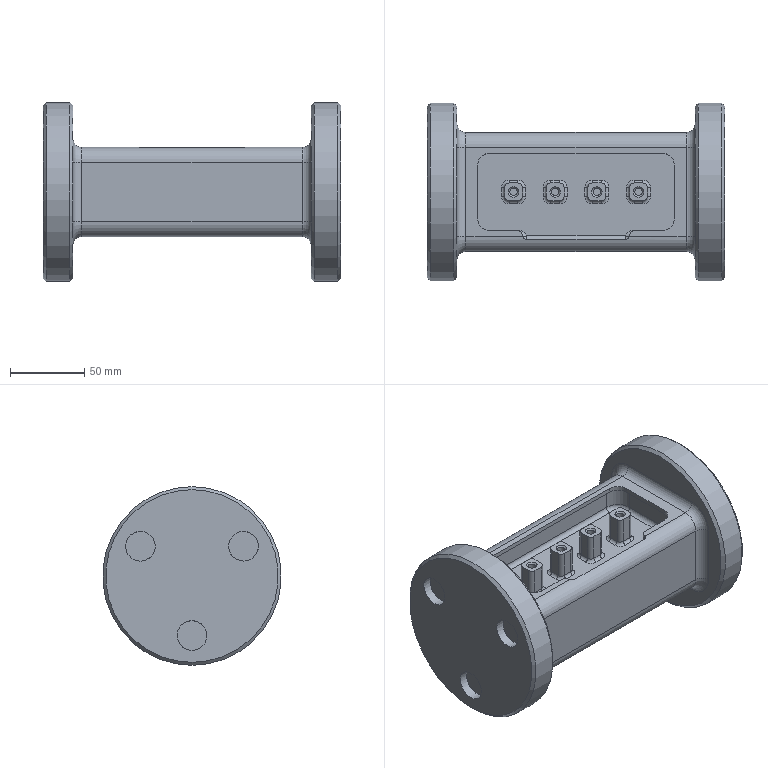NC program | NX | posted with a generic post | part box 200 x 120 x 120 mm
Lines 3125 to 4340 of 4340:
(CONTOUR_SURFACE_AREA , TOOL : PERSON_A_T_TOOL)
N6224 M6
N6226 G53
N6228 G17 G0 G90 X-24. Y-24. S3000 M3
N6230 G43 Z7. H0
N6232 Z1.
N6234 G94 G1 Z-9. F2500.
N6236 X-30.646
N6238 G3 X-38.875 Y-21. R11.134
N6240 G1 X-58.
N6242 G2 X-61. Y-18. R3.
N6244 G1 Y18.
N6246 G2 X-58. Y21. R3.
N6248 G1 X58.
N6250 G2 X61. Y18. R3.
N6252 G1 Y-18.
N6254 G2 X58. Y-21. R3.
N6256 G1 X38.875
N6258 G3 X30.646 Y-24. R11.134
N6260 G1 X24.
N6262 Z-9.367
N6264 X30.646
N6266 G2 X38.875 Y-21. R11.134
N6268 G1 X58.
N6270 G3 X61. Y-18. R3.
N6272 G1 Y18.
N6274 G3 X58. Y21. R3.
N6276 G1 X-58.
N6278 G3 X-61. Y18. R3.
N6280 G1 Y-18.
N6282 G3 X-58. Y-21. R3.
N6284 G1 X-38.875
N6286 G2 X-30.646 Y-24. R11.134
N6288 G1 X-24.
N6290 Z-9.733
N6292 X-30.646
N6294 G3 X-38.875 Y-21. R11.134
N6296 G1 X-58.
N6298 G2 X-61. Y-18. R3.
N6300 G1 Y18.
N6302 G2 X-58. Y21. R3.
N6304 G1 X58.
N6306 G2 X61. Y18. R3.
N6308 G1 Y-18.
N6310 G2 X58. Y-21. R3.
N6312 G1 X38.875
N6314 G3 X30.646 Y-24. R11.134
N6316 G1 X24.
N6318 Z-10.1
N6320 X30.646
N6322 G2 X38.875 Y-21. R11.134
N6324 G1 X58.
N6326 G3 X61. Y-18. R3.
N6328 G1 Y18.
N6330 G3 X58. Y21. R3.
N6332 G1 X-58.
N6334 G3 X-61. Y18. R3.
N6336 G1 Y-18.
N6338 G3 X-58. Y-21. R3.
N6340 G1 X-38.875
N6342 G2 X-30.646 Y-24. R11.134
N6344 G1 X-24.
N6346 Z-10.467
N6348 X-30.646
N6350 G3 X-38.875 Y-21. R11.134
N6352 G1 X-58.
N6354 G2 X-61. Y-18. R3.
N6356 G1 Y18.
N6358 G2 X-58. Y21. R3.
N6360 G1 X58.
N6362 G2 X61. Y18. R3.
N6364 G1 Y-18.
N6366 G2 X58. Y-21. R3.
N6368 G1 X38.875
N6370 G3 X30.646 Y-24. R11.134
N6372 G1 X24.
N6374 Z-10.833
N6376 X30.646
N6378 G2 X38.875 Y-21. R11.134
N6380 G1 X58.
N6382 G3 X61. Y-18. R3.
N6384 G1 Y18.
N6386 G3 X58. Y21. R3.
N6388 G1 X-58.
N6390 G3 X-61. Y18. R3.
N6392 G1 Y-18.
N6394 G3 X-58. Y-21. R3.
N6396 G1 X-38.875
N6398 G2 X-30.646 Y-24. R11.134
N6400 G1 X-24.
N6402 Z-11.2
N6404 X-30.646
N6406 G3 X-38.875 Y-21. R11.133
N6408 G1 X-58.
N6410 G2 X-61. Y-18. R3.
N6412 G1 Y18.
N6414 G2 X-58. Y21. R3.
N6416 G1 X58.
N6418 G2 X61. Y18. R3.
N6420 G1 Y-18.
N6422 G2 X58. Y-21. R3.
N6424 G1 X38.875
N6426 G3 X30.646 Y-24. R11.133
N6428 G1 X24.
N6430 Z-11.567
N6432 X30.646
N6434 G2 X38.875 Y-21. R11.133
N6436 G1 X58.
N6438 G3 X61. Y-18. R3.
N6440 G1 Y18.
N6442 G3 X58. Y21. R3.
N6444 G1 X-58.
N6446 G3 X-61. Y18. R3.
N6448 G1 Y-18.
N6450 G3 X-58. Y-21. R3.
N6452 G1 X-38.875
N6454 G2 X-30.646 Y-24. R11.134
N6456 G1 X-24.
N6458 Z-11.933
N6460 X-30.646
N6462 G3 X-38.875 Y-21. R11.134
N6464 G1 X-58.
N6466 G2 X-61. Y-18. R3.
N6468 G1 Y18.
N6470 G2 X-58. Y21. R3.
N6472 G1 X58.
N6474 G2 X61. Y18. R3.
N6476 G1 Y-18.
N6478 G2 X58. Y-21. R3.
N6480 G1 X38.875
N6482 G3 X30.646 Y-24. R11.134
N6484 G1 X24.
N6486 Z-12.3
N6488 X30.646
N6490 G2 X38.875 Y-21. R11.134
N6492 G1 X58.
N6494 G3 X61. Y-18. R3.
N6496 G1 Y18.
N6498 G3 X58. Y21. R3.
N6500 G1 X-58.
N6502 G3 X-61. Y18. R3.
N6504 G1 Y-18.
N6506 G3 X-58. Y-21. R3.
N6508 G1 X-38.875
N6510 G2 X-30.646 Y-24. R11.134
N6512 G1 X-24.
N6514 Z-12.667
N6516 X-30.646
N6518 G3 X-38.875 Y-21. R11.134
N6520 G1 X-58.
N6522 G2 X-61. Y-18. R3.
N6524 G1 Y18.
N6526 G2 X-58. Y21. R3.
N6528 G1 X58.
N6530 G2 X61. Y18. R3.
N6532 G1 Y-18.
N6534 G2 X58. Y-21. R3.
N6536 G1 X38.875
N6538 G3 X30.646 Y-24. R11.133
N6540 G1 X24.
N6542 Z-13.033
N6544 X30.646
N6546 G2 X38.875 Y-21. R11.134
N6548 G1 X58.
N6550 G3 X61. Y-18. R3.
N6552 G1 Y18.
N6554 G3 X58. Y21. R3.
N6556 G1 X-58.
N6558 G3 X-61. Y18. R3.
N6560 G1 Y-18.
N6562 G3 X-58. Y-21. R3.
N6564 G1 X-38.875
N6566 G2 X-30.646 Y-24. R11.134
N6568 G1 X-24.
N6570 Z-13.4
N6572 X-30.646
N6574 G3 X-38.875 Y-21. R11.133
N6576 G1 X-58.
N6578 G2 X-61. Y-18. R3.
N6580 G1 Y18.
N6582 G2 X-58. Y21. R3.
N6584 G1 X58.
N6586 G2 X61. Y18. R3.
N6588 G1 Y-18.
N6590 G2 X58. Y-21. R3.
N6592 G1 X38.875
N6594 G3 X30.646 Y-24. R11.133
N6596 G1 X24.
N6598 Z-13.767
N6600 X30.646
N6602 G2 X38.875 Y-21. R11.133
N6604 G1 X58.
N6606 G3 X61. Y-18. R3.
N6608 G1 Y18.
N6610 G3 X58. Y21. R3.
N6612 G1 X-58.
N6614 G3 X-61. Y18. R3.
N6616 G1 Y-18.
N6618 G3 X-58. Y-21. R3.
N6620 G1 X-38.875
N6622 G2 X-30.646 Y-24. R11.134
N6624 G1 X-24.
N6626 Z-14.133
N6628 X-30.646
N6630 G3 X-38.875 Y-21. R11.134
N6632 G1 X-58.
N6634 G2 X-61. Y-18. R3.
N6636 G1 Y18.
N6638 G2 X-58. Y21. R3.
N6640 G1 X58.
N6642 G2 X61. Y18. R3.
N6644 G1 Y-18.
N6646 G2 X58. Y-21. R3.
N6648 G1 X38.875
N6650 G3 X30.646 Y-24. R11.134
N6652 G1 X24.
N6654 Z-14.5
N6656 X30.646
N6658 G2 X38.875 Y-21. R11.134
N6660 G1 X58.
N6662 G3 X61. Y-18. R3.
N6664 G1 Y18.
N6666 G3 X58. Y21. R3.
N6668 G1 X-58.
N6670 G3 X-61. Y18. R3.
N6672 G1 Y-18.
N6674 G3 X-58. Y-21. R3.
N6676 G1 X-38.875
N6678 G2 X-30.646 Y-24. R11.134
N6680 G1 X-24.
N6682 Z-14.867
N6684 X-30.646
N6686 G3 X-38.875 Y-21. R11.134
N6688 G1 X-58.
N6690 G2 X-61. Y-18. R3.
N6692 G1 Y18.
N6694 G2 X-58. Y21. R3.
N6696 G1 X58.
N6698 G2 X61. Y18. R3.
N6700 G1 Y-18.
N6702 G2 X58. Y-21. R3.
N6704 G1 X38.875
N6706 G3 X30.646 Y-24. R11.134
N6708 G1 X24.
N6710 Z-15.233
N6712 X30.646
N6714 G2 X38.875 Y-21. R11.134
N6716 G1 X58.
N6718 G3 X61. Y-18. R3.
N6720 G1 Y18.
N6722 G3 X58. Y21. R3.
N6724 G1 X-58.
N6726 G3 X-61. Y18. R3.
N6728 G1 Y-18.
N6730 G3 X-58. Y-21. R3.
N6732 G1 X-38.875
N6734 G2 X-30.646 Y-24. R11.134
N6736 G1 X-24.
N6738 Z-15.6
N6740 X-30.646
N6742 G3 X-38.875 Y-21. R11.134
N6744 G1 X-58.
N6746 G2 X-61. Y-18. R3.
N6748 G1 Y18.
N6750 G2 X-58. Y21. R3.
N6752 G1 X58.
N6754 G2 X61. Y18. R3.
N6756 G1 Y-18.
N6758 G2 X58. Y-21. R3.
N6760 G1 X38.875
N6762 G3 X30.646 Y-24. R11.134
N6764 G1 X24.
N6766 Z-15.967
N6768 X30.646
N6770 G2 X38.875 Y-21. R11.134
N6772 G1 X58.
N6774 G3 X61. Y-18. R3.
N6776 G1 Y18.
N6778 G3 X58. Y21. R3.
N6780 G1 X-58.
N6782 G3 X-61. Y18. R3.
N6784 G1 Y-18.
N6786 G3 X-58. Y-21. R3.
N6788 G1 X-38.875
N6790 G2 X-30.646 Y-24. R11.134
N6792 G1 X-24.
N6794 Z-16.333
N6796 X-30.646
N6798 G3 X-38.875 Y-21. R11.134
N6800 G1 X-58.
N6802 G2 X-61. Y-18. R3.
N6804 G1 Y18.
N6806 G2 X-58. Y21. R3.
N6808 G1 X58.
N6810 G2 X61. Y18. R3.
N6812 G1 Y-18.
N6814 G2 X58. Y-21. R3.
N6816 G1 X38.875
N6818 G3 X30.646 Y-24. R11.134
N6820 G1 X24.
N6822 Z-16.7
N6824 X30.646
N6826 G2 X38.875 Y-21. R11.134
N6828 G1 X58.
N6830 G3 X61. Y-18. R3.
N6832 G1 Y18.
N6834 G3 X58. Y21. R3.
N6836 G1 X-58.
N6838 G3 X-61. Y18. R3.
N6840 G1 Y-18.
N6842 G3 X-58. Y-21. R3.
N6844 G1 X-38.875
N6846 G2 X-30.646 Y-24. R11.134
N6848 G1 X-24.
N6850 Y-23.999 Z-17.067
N6852 X-30.646
N6854 G3 X-38.875 Y-20.999 R11.134
N6856 G1 X-58.
N6858 G2 X-60.999 Y-18. R2.999
N6860 G1 Y18.
N6862 G2 X-58. Y20.999 R2.999
N6864 G1 X58.
N6866 G2 X60.999 Y18. R2.999
N6868 G1 Y-18.
N6870 G2 X58. Y-20.999 R2.999
N6872 G1 X38.875
N6874 G3 X30.646 Y-23.999 R11.134
N6876 G1 X24.
N6878 Y-23.969 Z-17.433
N6880 X30.634
N6882 G2 X38.875 Y-20.969 R11.165
N6884 G1 X58.
N6886 G3 X60.969 Y-18. R2.969
N6888 G1 Y18.
N6890 G3 X58. Y20.969 R2.969
N6892 G1 X-58.
N6894 G3 X-60.969 Y18. R2.969
N6896 G1 Y-18.
N6898 G3 X-58. Y-20.969 R2.969
N6900 G1 X-38.875
N6902 G2 X-30.634 Y-23.969 R11.165
N6904 G1 X-24.
N6906 Y-23.891 Z-17.8
N6908 X-30.603
N6910 G3 X-38.875 Y-20.891 R11.243
N6912 G1 X-58.
N6914 G2 X-60.891 Y-18. R2.891
N6916 G1 Y18.
N6918 G2 X-58. Y20.891 R2.891
N6920 G1 X58.
N6922 G2 X60.891 Y18. R2.891
N6924 G1 Y-18.
N6926 G2 X58. Y-20.891 R2.891
N6928 G1 X38.875
N6930 G3 X30.603 Y-23.891 R11.243
N6932 G1 X24.
N6934 Y-23.764 Z-18.167
N6936 X30.553
N6938 G2 X38.875 Y-20.764 R11.371
N6940 G1 X58.
N6942 G3 X60.764 Y-18. R2.764
N6944 G1 Y18.
N6946 G3 X58. Y20.764 R2.764
N6948 G1 X-58.
N6950 G3 X-60.764 Y18. R2.764
N6952 G1 Y-18.
N6954 G3 X-58. Y-20.764 R2.764
N6956 G1 X-38.875
N6958 G2 X-30.553 Y-23.764 R11.371
N6960 G1 X-24.
N6962 Y-23.679 Z-18.35
N6964 Y-23.579 Z-18.533
N6966 X-30.481
N6968 G3 X-38.875 Y-20.579 R11.558
N6970 G1 X-58.
N6972 G2 X-60.579 Y-18. R2.579
N6974 G1 Y18.
N6976 G2 X-58. Y20.579 R2.579
N6978 G1 X58.
N6980 G2 X60.579 Y18. R2.579
N6982 G1 Y-18.
N6984 G2 X58. Y-20.579 R2.579
N6986 G1 X38.875
N6988 G3 X30.481 Y-23.579 R11.558
N6990 G1 X24.
N6992 Y-23.46 Z-18.717
N6994 Y-23.322 Z-18.9
N6996 X30.381
N6998 G2 X38.875 Y-20.322 R11.816
N7000 G1 X58.
N7002 G3 X60.322 Y-18. R2.322
N7004 G1 Y18.
N7006 G3 X58. Y20.322 R2.322
N7008 G1 X-58.
N7010 G3 X-60.322 Y18. R2.322
N7012 G1 Y-18.
N7014 G3 X-58. Y-20.322 R2.322
N7016 G1 X-38.875
N7018 G2 X-30.381 Y-23.322 R11.816
N7020 G1 X-24.
N7022 Y-23.159 Z-19.083
N7024 Y-23.066 Z-19.175
N7026 Y-22.965 Z-19.267
N7028 X-30.246
N7030 G3 X-38.875 Y-19.965 R12.175
N7032 G1 X-58.
N7034 G2 X-59.965 Y-18. R1.965
N7036 G1 Y18.
N7038 G2 X-58. Y19.965 R1.965
N7040 G1 X58.
N7042 G2 X59.965 Y18. R1.965
N7044 G1 Y-18.
N7046 G2 X58. Y-19.965 R1.965
N7048 G1 X38.875
N7050 G3 X30.246 Y-22.965 R12.175
N7052 G1 X24.
N7054 Y-22.854 Z-19.358
N7056 Y-22.731 Z-19.45
N7058 Y-22.594 Z-19.542
N7060 Y-22.437 Z-19.633
N7062 X30.049
N7064 G2 X38.875 Y-19.437 R12.706
N7066 G1 X58.
N7068 G3 X59.437 Y-18. R1.437
N7070 G1 Y18.
N7072 G3 X58. Y19.437 R1.437
N7074 G1 X-58.
N7076 G3 X-59.437 Y18. R1.437
N7078 G1 Y-18.
N7080 G3 X-58. Y-19.437 R1.437
N7082 G1 X-38.875
N7084 G2 X-30.049 Y-22.437 R12.706
N7086 G1 X-24.
N7088 Y-22.35 Z-19.679
N7090 Y-22.255 Z-19.725
N7092 Y-22.033 Z-19.817
N7094 Y-21.736 Z-19.908
N7096 Y-21.522 Z-19.954
N7098 Y-21. Z-20.
N7100 X-28.25
N7102 X-29.313
N7104 X-29.578 Y-20.967
N7106 G3 X-36.75 Y-18.077 R14.082
N7108 G1 X-38.875 Y-18.
N7110 X-41. Y-18.005
N7112 X-49.5 Y-18.
N7114 X-53.75
N7116 X-55.875 Y-18.005
N7118 X-57.997 Y-17.998
N7120 X-57.998 Y-17.997
N7122 X-57.996 Y-17.998
N7124 X-57.998 Y-17.997
N7126 Y-17.998
N7128 X-57.991
N7130 X-57.988
N7132 X-57.987 Y-17.999
N7134 X-50.574 Y-18.
N7136 X-58. Y-17.965
N7138 Y9.
N7140 X-57.981 Y18.
N7142 X-57.987 Y17.999
N7144 X-57.991
N7146 X-57.993
N7148 X-57.998 Y17.998
N7150 X-57.996
N7152 X-57.998
N7154 X-57.997
N7156 X-57.998
N7158 Y17.991
N7160 X-58.
N7162 Y17.989
N7164 X-50.75 Y18.
N7166 X57.943
N7168 X57.999 Y17.993
N7170 X57.997 Y17.998
N7172 X57.998 Y17.996
N7174 X58. Y18.
N7176 X57.996 Y17.999
N7178 X57.998 Y17.997
N7180 X57.984 Y-17.999
N7182 X57.988 Y-17.998
N7184 X57.991
N7186 X57.998
N7188 X57.995
N7190 X57.998
N7192 Y-17.995
N7194 X57.997 Y-17.998
N7196 X57.998
N7198 Y-17.991
N7200 Y-17.988
N7202 X57.999 Y-17.984
N7204 X58. Y-17.911
N7206 X53.75 Y-18.
N7208 X49.5
N7210 X41. Y-18.005
N7212 X38.875 Y-18.
N7214 X36.75 Y-18.077
N7216 G3 X29.578 Y-20.967 R14.05
N7218 G1 X29.313 Y-21.
N7220 X24.
N7222 Z-17.
N7224 G0 Z7.
(CONTOUR_SURFACE_AREA_COPY , TOOL : PERSON_A_T_TOOL)
N7226 X-24. Y-26.
N7228 Z1.
N7230 Z-8.7
N7232 G1 Z-9.
N7234 X-58.
N7236 G2 X-66. Y-18. R8.
N7238 G1 Y18.
N7240 G2 X-58. Y26. R8.
N7242 G1 X58.
N7244 G2 X66. Y18. R8.
N7246 G1 Y-18.
N7248 G2 X58. Y-26. R8.
N7250 G1 X24.
N7252 Z-10.1
N7254 X58.
N7256 G3 X66. Y-18. R8.
N7258 G1 Y18.
N7260 G3 X58. Y26. R8.
N7262 G1 X-58.
N7264 G3 X-66. Y18. R8.
N7266 G1 Y-18.
N7268 G3 X-58. Y-26. R8.
N7270 G1 X-24.
N7272 Z-11.2
N7274 X-58.
N7276 G2 X-66. Y-18. R8.
N7278 G1 Y18.
N7280 G2 X-58. Y26. R8.
N7282 G1 X58.
N7284 G2 X66. Y18. R8.
N7286 G1 Y-18.
N7288 G2 X58. Y-26. R8.
N7290 G1 X24.
N7292 Z-12.3
N7294 X58.
N7296 G3 X66. Y-18. R8.
N7298 G1 Y18.
N7300 G3 X58. Y26. R8.
N7302 G1 X-58.
N7304 G3 X-66. Y18. R8.
N7306 G1 Y-18.
N7308 G3 X-58. Y-26. R8.
N7310 G1 X-24.
N7312 Z-13.4
N7314 X-58.
N7316 G2 X-66. Y-18. R8.
N7318 G1 Y18.
N7320 G2 X-58. Y26. R8.
N7322 G1 X58.
N7324 G2 X66. Y18. R8.
N7326 G1 Y-18.
N7328 G2 X58. Y-26. R8.
N7330 G1 X24.
N7332 Z-14.5
N7334 X58.
N7336 G3 X66. Y-18. R8.
N7338 G1 Y18.
N7340 G3 X58. Y26. R8.
N7342 G1 X-58.
N7344 G3 X-66. Y18. R8.
N7346 G1 Y-18.
N7348 G3 X-58. Y-26. R8.
N7350 G1 X-24.
N7352 Z-15.6
N7354 X-58.
N7356 G2 X-66. Y-18. R8.
N7358 G1 Y18.
N7360 G2 X-58. Y26. R8.
N7362 G1 X58.
N7364 G2 X66. Y18. R8.
N7366 G1 Y-18.
N7368 G2 X58. Y-26. R8.
N7370 G1 X24.
N7372 Z-16.7
N7374 X58.
N7376 G3 X66. Y-18. R8.
N7378 G1 Y18.
N7380 G3 X58. Y26. R8.
N7382 G1 X-58.
N7384 G3 X-66. Y18. R8.
N7386 G1 Y-18.
N7388 G3 X-58. Y-26. R8.
N7390 G1 X-24.
N7392 Z-17.8
N7394 X-58.
N7396 G2 X-66. Y-18. R8.
N7398 G1 Y18.
N7400 G2 X-58. Y26. R8.
N7402 G1 X58.
N7404 G2 X66. Y18. R8.
N7406 G1 Y-18.
N7408 G2 X58. Y-26. R8.
N7410 G1 X24.
N7412 Z-18.9
N7414 X58.
N7416 G3 X66. Y-18. R8.
N7418 G1 Y18.
N7420 G3 X58. Y26. R8.
N7422 G1 X-58.
N7424 G3 X-66. Y18. R8.
N7426 G1 Y-18.
N7428 G3 X-58. Y-26. R8.
N7430 G1 X-24.
N7432 Z-20.
N7434 X-58.
N7436 G2 X-66. Y-18. R8.
N7438 G1 Y18.
N7440 G2 X-58. Y26. R8.
N7442 G1 X58.
N7444 G2 X66. Y18. R8.
N7446 G1 Y-18.
N7448 G2 X58. Y-26. R8.
N7450 G1 X24.
N7452 Z-19.7
N7454 G0 Z1.
(CONTOUR_SURFACE_AREA_COPY_1 , TOOL : PERSON_A_T_TOOL)
N7456 Z7.
N7458 X-24. Y-24.
N7460 Z1.
N7462 G1 Z-9.
N7464 X-30.646
N7466 G3 X-38.875 Y-21. R11.134
N7468 G1 X-58.
N7470 G2 X-61. Y-18. R3.
N7472 G1 Y18.
N7474 G2 X-58. Y21. R3.
N7476 G1 X58.
N7478 G2 X61. Y18. R3.
N7480 G1 Y-18.
N7482 G2 X58. Y-21. R3.
N7484 G1 X38.875
N7486 G3 X30.646 Y-24. R11.134
N7488 G1 X24.
N7490 Z-10.54
N7492 X30.646
N7494 G2 X38.875 Y-21. R11.134
N7496 G1 X58.
N7498 G3 X61. Y-18. R3.
N7500 G1 Y18.
N7502 G3 X58. Y21. R3.
N7504 G1 X-58.
N7506 G3 X-61. Y18. R3.
N7508 G1 Y-18.
N7510 G3 X-58. Y-21. R3.
N7512 G1 X-38.875
N7514 G2 X-30.646 Y-24. R11.134
N7516 G1 X-24.
N7518 Z-12.08
N7520 X-30.646
N7522 G3 X-38.875 Y-21. R11.133
N7524 G1 X-58.
N7526 G2 X-61. Y-18. R3.
N7528 G1 Y18.
N7530 G2 X-58. Y21. R3.
N7532 G1 X58.
N7534 G2 X61. Y18. R3.
N7536 G1 Y-18.
N7538 G2 X58. Y-21. R3.
N7540 G1 X38.875
N7542 G3 X30.646 Y-24. R11.134
N7544 G1 X24.
N7546 Z-13.62
N7548 X30.646
N7550 G2 X38.875 Y-21. R11.134
N7552 G1 X58.
N7554 G3 X61. Y-18. R3.
N7556 G1 Y18.
N7558 G3 X58. Y21. R3.
N7560 G1 X-58.
N7562 G3 X-61. Y18. R3.
N7564 G1 Y-18.
N7566 G3 X-58. Y-21. R3.
N7568 G1 X-38.875
N7570 G2 X-30.646 Y-24. R11.134
N7572 G1 X-24.
N7574 Z-15.16
N7576 X-30.646
N7578 G3 X-38.875 Y-21. R11.134
N7580 G1 X-58.
N7582 G2 X-61. Y-18. R3.
N7584 G1 Y18.
N7586 G2 X-58. Y21. R3.
N7588 G1 X58.
N7590 G2 X61. Y18. R3.
N7592 G1 Y-18.
N7594 G2 X58. Y-21. R3.
N7596 G1 X38.875
N7598 G3 X30.646 Y-24. R11.134
N7600 G1 X24.
N7602 Z-16.7
N7604 X30.646
N7606 G2 X38.875 Y-21. R11.134
N7608 G1 X58.
N7610 G3 X61. Y-18. R3.
N7612 G1 Y18.
N7614 G3 X58. Y21. R3.
N7616 G1 X-58.
N7618 G3 X-61. Y18. R3.
N7620 G1 Y-18.
N7622 G3 X-58. Y-21. R3.
N7624 G1 X-38.875
N7626 G2 X-30.646 Y-24. R11.134
N7628 G1 X-24.
N7630 Z1.
N7632 G0 Z7.
(CONTOUR_SURFACE_AREA_COPY_1_COPY , TOOL : PERSON_A_T_TOOL)
N7634 Z1.
N7636 G1 Z-16.7
N7638 X-30.646
N7640 G3 X-38.875 Y-21. R11.134
N7642 G1 X-58.
N7644 G2 X-61. Y-18. R3.
N7646 G1 Y18.
N7648 G2 X-58. Y21. R3.
N7650 G1 X58.
N7652 G2 X61. Y18. R3.
N7654 G1 Y-18.
N7656 G2 X58. Y-21. R3.
N7658 G1 X38.875
N7660 G3 X30.646 Y-24. R11.134
N7662 G1 X24.
N7664 Z-16.81
N7666 X30.646
N7668 G2 X38.875 Y-21. R11.134
N7670 G1 X58.
N7672 G3 X61. Y-18. R3.
N7674 G1 Y18.
N7676 G3 X58. Y21. R3.
N7678 G1 X-58.
N7680 G3 X-61. Y18. R3.
N7682 G1 Y-18.
N7684 G3 X-58. Y-21. R3.
N7686 G1 X-38.875
N7688 G2 X-30.646 Y-24. R11.134
N7690 G1 X-24.
N7692 Z-16.92
N7694 X-30.646
N7696 G3 X-38.875 Y-21. R11.134
N7698 G1 X-58.
N7700 G2 X-61. Y-18. R3.
N7702 G1 Y18.
N7704 G2 X-58. Y21. R3.
N7706 G1 X58.
N7708 G2 X61. Y18. R3.
N7710 G1 Y-18.
N7712 G2 X58. Y-21. R3.
N7714 G1 X38.875
N7716 G3 X30.646 Y-24. R11.134
N7718 G1 X24.
N7720 Z-17.03
N7722 X30.646
N7724 G2 X38.875 Y-21. R11.134
N7726 G1 X58.
N7728 G3 X61. Y-18. R3.
N7730 G1 Y18.
N7732 G3 X58. Y21. R3.
N7734 G1 X-58.
N7736 G3 X-61. Y18. R3.
N7738 G1 Y-18.
N7740 G3 X-58. Y-21. R3.
N7742 G1 X-38.875
N7744 G2 X-30.646 Y-24. R11.134
N7746 G1 X-24.
N7748 Y-23.997 Z-17.14
N7750 X-30.645
N7752 G3 X-38.875 Y-20.997 R11.137
N7754 G1 X-58.
N7756 G2 X-60.997 Y-18. R2.997
N7758 G1 Y18.
N7760 G2 X-58. Y20.997 R2.997
N7762 G1 X58.
N7764 G2 X60.997 Y18. R2.997
N7766 G1 Y-18.
N7768 G2 X58. Y-20.997 R2.997
N7770 G1 X38.875
N7772 G3 X30.645 Y-23.997 R11.137
N7774 G1 X24.
N7776 Y-23.99 Z-17.25
N7778 X30.633
N7780 G2 X38.875 Y-20.99 R11.18
N7782 G1 X58.
N7784 G3 X60.99 Y-18. R2.99
N7786 G1 Y18.
N7788 G3 X58. Y20.99 R2.99
N7790 G1 X-58.
N7792 G3 X-60.99 Y18. R2.99
N7794 G1 Y-18.
N7796 G3 X-58. Y-20.99 R2.99
N7798 G1 X-38.875
N7800 G2 X-30.633 Y-23.99 R11.18
N7802 G1 X-24.
N7804 Y-23.978 Z-17.36
N7806 X-30.638
N7808 G3 X-38.875 Y-20.978 R11.155
N7810 G1 X-58.
N7812 G2 X-60.978 Y-18. R2.978
N7814 G1 Y18.
N7816 G2 X-58. Y20.978 R2.978
N7818 G1 X58.
N7820 G2 X60.978 Y18. R2.978
N7822 G1 Y-18.
N7824 G2 X58. Y-20.978 R2.978
N7826 G1 X38.875
N7828 G3 X30.638 Y-23.978 R11.155
N7830 G1 X24.
N7832 Y-23.963 Z-17.47
N7834 X30.632
N7836 G2 X38.875 Y-20.963 R11.171
N7838 G1 X58.
N7840 G3 X60.963 Y-18. R2.963
N7842 G1 Y18.
N7844 G3 X58. Y20.963 R2.963
N7846 G1 X-58.
N7848 G3 X-60.963 Y18. R2.963
N7850 G1 Y-18.
N7852 G3 X-58. Y-20.963 R2.963
N7854 G1 X-38.875
N7856 G2 X-30.632 Y-23.963 R11.171
N7858 G1 X-24.
N7860 Y-23.943 Z-17.58
N7862 X-30.624
N7864 G3 X-38.875 Y-20.943 R11.191
N7866 G1 X-58.
N7868 G2 X-60.943 Y-18. R2.943
N7870 G1 Y18.
N7872 G2 X-58. Y20.943 R2.943
N7874 G1 X58.
N7876 G2 X60.943 Y18. R2.943
N7878 G1 Y-18.
N7880 G2 X58. Y-20.943 R2.943
N7882 G1 X38.875
N7884 G3 X30.624 Y-23.943 R11.191
N7886 G1 X24.
N7888 Y-23.92 Z-17.69
N7890 X30.614
N7892 G2 X38.875 Y-20.92 R11.214
N7894 G1 X58.
N7896 G3 X60.92 Y-18. R2.92
N7898 G1 Y18.
N7900 G3 X58. Y20.92 R2.92
N7902 G1 X-58.
N7904 G3 X-60.92 Y18. R2.92
N7906 G1 Y-18.
N7908 G3 X-58. Y-20.92 R2.92
N7910 G1 X-38.875
N7912 G2 X-30.614 Y-23.92 R11.214
N7914 G1 X-24.
N7916 Y-23.891 Z-17.8
N7918 X-30.603
N7920 G3 X-38.875 Y-20.891 R11.243
N7922 G1 X-58.
N7924 G2 X-60.891 Y-18. R2.891
N7926 G1 Y18.
N7928 G2 X-58. Y20.891 R2.891
N7930 G1 X58.
N7932 G2 X60.891 Y18. R2.891
N7934 G1 Y-18.
N7936 G2 X58. Y-20.891 R2.891
N7938 G1 X38.875
N7940 G3 X30.603 Y-23.891 R11.243
N7942 G1 X24.
N7944 Y-23.859 Z-17.91
N7946 X30.59
N7948 G2 X38.875 Y-20.859 R11.276
N7950 G1 X58.
N7952 G3 X60.859 Y-18. R2.859
N7954 G1 Y18.
N7956 G3 X58. Y20.859 R2.859
N7958 G1 X-58.
N7960 G3 X-60.859 Y18. R2.859
N7962 G1 Y-18.
N7964 G3 X-58. Y-20.859 R2.859
N7966 G1 X-38.875
N7968 G2 X-30.59 Y-23.859 R11.276
N7970 G1 X-24.
N7972 Y-23.821 Z-18.02
N7974 X-30.575
N7976 G3 X-38.875 Y-20.821 R11.315
N7978 G1 X-58.
N7980 G2 X-60.821 Y-18. R2.821
N7982 G1 Y18.
N7984 G2 X-58. Y20.821 R2.821
N7986 G1 X58.
N7988 G2 X60.821 Y18. R2.821
N7990 G1 Y-18.
N7992 G2 X58. Y-20.821 R2.821
N7994 G1 X38.875
N7996 G3 X30.575 Y-23.821 R11.315
N7998 G1 X24.
N8000 Y-23.779 Z-18.13
N8002 X30.559
N8004 G2 X38.875 Y-20.779 R11.356
N8006 G1 X58.
N8008 G3 X60.779 Y-18. R2.779
N8010 G1 Y18.
N8012 G3 X58. Y20.779 R2.779
N8014 G1 X-58.
N8016 G3 X-60.779 Y18. R2.779
N8018 G1 Y-18.
N8020 G3 X-58. Y-20.779 R2.779
N8022 G1 X-38.875
N8024 G2 X-30.559 Y-23.779 R11.356
N8026 G1 X-24.
N8028 Y-23.732 Z-18.24
N8030 X-30.54
N8032 G3 X-38.875 Y-20.732 R11.404
N8034 G1 X-58.
N8036 G2 X-60.732 Y-18. R2.732
N8038 G1 Y18.
N8040 G2 X-58. Y20.732 R2.732
N8042 G1 X58.
N8044 G2 X60.732 Y18. R2.732
N8046 G1 Y-18.
N8048 G2 X58. Y-20.732 R2.732
N8050 G1 X38.875
N8052 G3 X30.54 Y-23.732 R11.404
N8054 G1 X24.
N8056 Y-23.679 Z-18.35
N8058 X30.52
N8060 G2 X38.875 Y-20.679 R11.457
N8062 G1 X58.
N8064 G3 X60.679 Y-18. R2.679
N8066 G1 Y18.
N8068 G3 X58. Y20.679 R2.679
N8070 G1 X-58.
N8072 G3 X-60.679 Y18. R2.679
N8074 G1 Y-18.
N8076 G3 X-58. Y-20.679 R2.679
N8078 G1 X-38.875
N8080 G2 X-30.52 Y-23.679 R11.457
N8082 G1 X-24.
N8084 Y-23.621 Z-18.46
N8086 X-30.497
N8088 G3 X-38.875 Y-20.621 R11.515
N8090 G1 X-58.
N8092 G2 X-60.621 Y-18. R2.621
N8094 G1 Y18.
N8096 G2 X-58. Y20.621 R2.621
N8098 G1 X58.
N8100 G2 X60.621 Y18. R2.621
N8102 G1 Y-18.
N8104 G2 X58. Y-20.621 R2.621
N8106 G1 X38.875
N8108 G3 X30.497 Y-23.621 R11.515
N8110 G1 X24.
N8112 Y-23.556 Z-18.57
N8114 X30.472
N8116 G2 X38.875 Y-20.556 R11.581
N8118 G1 X58.
N8120 G3 X60.556 Y-18. R2.556
N8122 G1 Y18.
N8124 G3 X58. Y20.556 R2.556
N8126 G1 X-58.
N8128 G3 X-60.556 Y18. R2.556
N8130 G1 Y-18.
N8132 G3 X-58. Y-20.556 R2.556
N8134 G1 X-38.875
N8136 G2 X-30.472 Y-23.556 R11.581
N8138 G1 X-24.
N8140 Y-23.485 Z-18.68
N8142 X-30.445
N8144 G3 X-38.875 Y-20.485 R11.651
N8146 G1 X-58.
N8148 G2 X-60.485 Y-18. R2.485
N8150 G1 Y18.
N8152 G2 X-58. Y20.485 R2.485
N8154 G1 X58.
N8156 G2 X60.485 Y18. R2.485
N8158 G1 Y-18.
N8160 G2 X58. Y-20.485 R2.485
N8162 G1 X38.875
N8164 G3 X30.445 Y-23.485 R11.651
N8166 G1 X24.
N8168 Y-23.407 Z-18.79
N8170 X30.414
N8172 G2 X38.875 Y-20.407 R11.73
N8174 G1 X58.
N8176 G3 X60.407 Y-18. R2.407
N8178 G1 Y18.
N8180 G3 X58. Y20.407 R2.407
N8182 G1 X-58.
N8184 G3 X-60.407 Y18. R2.407
N8186 G1 Y-18.
N8188 G3 X-58. Y-20.407 R2.407
N8190 G1 X-38.875
N8192 G2 X-30.414 Y-23.407 R11.73
N8194 G1 X-24.
N8196 Y-23.322 Z-18.9
N8198 X-30.381
N8200 G3 X-38.875 Y-20.322 R11.816
N8202 G1 X-58.
N8204 G2 X-60.322 Y-18. R2.322
N8206 G1 Y18.
N8208 G2 X-58. Y20.322 R2.322
N8210 G1 X58.
N8212 G2 X60.322 Y18. R2.322
N8214 G1 Y-18.
N8216 G2 X58. Y-20.322 R2.322
N8218 G1 X38.875
N8220 G3 X30.381 Y-23.322 R11.816
N8222 G1 X24.
N8224 Y-23.227 Z-19.01
N8226 X30.345
N8228 G2 X38.875 Y-20.227 R11.911
N8230 G1 X58.
N8232 G3 X60.227 Y-18. R2.227
N8234 G1 Y18.
N8236 G3 X58. Y20.227 R2.227
N8238 G1 X-58.
N8240 G3 X-60.227 Y18. R2.227
N8242 G1 Y-18.
N8244 G3 X-58. Y-20.227 R2.227
N8246 G1 X-38.875
N8248 G2 X-30.345 Y-23.227 R11.911
N8250 G1 X-24.
N8252 Y-23.123 Z-19.12
N8254 X-30.305
N8256 G3 X-38.875 Y-20.123 R12.017
N8258 G1 X-58.
N8260 G2 X-60.123 Y-18. R2.123
N8262 G1 Y18.
N8264 G2 X-58. Y20.123 R2.123
N8266 G1 X58.
N8268 G2 X60.123 Y18. R2.123
N8270 G1 Y-18.
N8272 G2 X58. Y-20.123 R2.123
N8274 G1 X38.875
N8276 G3 X30.305 Y-23.123 R12.017
N8278 G1 X24.
N8280 Y-23.007 Z-19.23
N8282 X30.261
N8284 G2 X38.875 Y-20.007 R12.133
N8286 G1 X58.
N8288 G3 X60.007 Y-18. R2.007
N8290 G1 Y18.
N8292 G3 X58. Y20.007 R2.007
N8294 G1 X-58.
N8296 G3 X-60.007 Y18. R2.007
N8298 G1 Y-18.
N8300 G3 X-58. Y-20.007 R2.007
N8302 G1 X-38.875
N8304 G2 X-30.261 Y-23.007 R12.133
N8306 G1 X-24.
N8308 Y-22.877 Z-19.34
N8310 X-30.213
N8312 G3 X-38.875 Y-19.877 R12.263
N8314 G1 X-58.
N8316 G2 X-59.877 Y-18. R1.877
N8318 G1 Y18.
N8320 G2 X-58. Y19.877 R1.877
N8322 G1 X58.
N8324 G2 X59.877 Y18. R1.877
N8326 G1 Y-18.
N8328 G2 X58. Y-19.877 R1.877
N8330 G1 X38.875
N8332 G3 X30.213 Y-22.877 R12.263
N8334 G1 X24.
N8336 Y-22.731 Z-19.45
N8338 X30.158
N8340 G2 X38.875 Y-19.731 R12.411
N8342 G1 X58.
N8344 G3 X59.731 Y-18. R1.731
N8346 G1 Y18.
N8348 G3 X58. Y19.731 R1.731
N8350 G1 X-58.
N8352 G3 X-59.731 Y18. R1.731
N8354 G1 Y-18.
N8356 G3 X-58. Y-19.731 R1.731
N8358 G1 X-38.875
N8360 G2 X-30.158 Y-22.731 R12.411
N8362 G1 X-24.
N8364 Y-22.651 Z-19.505
N8366 Y-22.564 Z-19.56
N8368 X-30.096
N8370 G3 X-38.875 Y-19.564 R12.579
N8372 G1 X-58.
N8374 G2 X-59.564 Y-18. R1.564
N8376 G1 Y18.
N8378 G2 X-58. Y19.564 R1.564
N8380 G1 X58.
N8382 G2 X59.564 Y18. R1.564
N8384 G1 Y-18.
N8386 G2 X58. Y-19.564 R1.564
N8388 G1 X38.875
N8390 G3 X30.096 Y-22.564 R12.579
N8392 G1 X24.
N8394 Y-22.47 Z-19.615
N8396 Y-22.368 Z-19.67
N8398 X30.023
N8400 G2 X38.875 Y-19.368 R12.776
N8402 G1 X58.
N8404 G3 X59.368 Y-18. R1.368
N8406 G1 Y18.
N8408 G3 X58. Y19.368 R1.368
N8410 G1 X-58.
N8412 G3 X-59.368 Y18. R1.368
N8414 G1 Y-18.
N8416 G3 X-58. Y-19.368 R1.368
N8418 G1 X-38.875
N8420 G2 X-30.023 Y-22.368 R12.776
N8422 G1 X-24.
N8424 Y-22.255 Z-19.725
N8426 Y-22.128 Z-19.78
N8428 X-29.936
N8430 G3 X-36.75 Y-19.209 R12.872
N8432 G1 X-38.875 Y-19.128
N8434 X-58.
N8436 G2 X-59.128 Y-18. R1.128
N8438 G1 Y18.
N8440 G2 X-58. Y19.128 R1.128
N8442 G1 X58.
N8444 G2 X59.128 Y18. R1.128
N8446 G1 Y-18.
N8448 G2 X58. Y-19.128 R1.128
N8450 G1 X38.875
N8452 X36.75 Y-19.209
N8454 G3 X29.936 Y-22.128 R12.872
N8456 G1 X24.
N8458 Y-21.981 Z-19.835
N8460 Y-21.898 Z-19.863
N8462 Y-21.805 Z-19.89
N8464 X29.819
N8466 G2 X36.75 Y-18.884 R13.195
N8468 G1 X38.875 Y-18.805
N8470 X58.
N8472 G3 X58.805 Y-18. R0.805
N8474 G1 Y18.
N8476 G3 X58. Y18.805 R0.805
N8478 G1 X-58.
N8480 G3 X-58.805 Y18. R0.805
N8482 G1 Y-18.
N8484 G3 X-58. Y-18.805 R0.805
N8486 G1 X-38.875
N8488 X-36.75 Y-18.884
N8490 G2 X-29.819 Y-21.805 R13.195
N8492 G1 X-24.
N8494 Y-21.699 Z-19.918
N8496 Y-21.572 Z-19.945
N8498 Y-21.405 Z-19.973
N8500 Y-21. Z-20.
N8502 X-28.25
N8504 X-29.313
N8506 X-29.578 Y-20.967
N8508 G3 X-36.75 Y-18.077 R14.082
N8510 G1 X-38.875 Y-18.
N8512 X-41. Y-18.005
N8514 X-49.5 Y-18.
N8516 X-53.75
N8518 X-55.875 Y-18.005
N8520 X-57.997 Y-17.998
N8522 X-57.998 Y-17.997
N8524 X-57.996 Y-17.998
N8526 X-57.998 Y-17.997
N8528 Y-17.998
N8530 X-57.991
N8532 X-57.988
N8534 X-57.987 Y-17.999
N8536 X-50.574 Y-18.
N8538 X-58. Y-17.965
N8540 Y9.
N8542 X-57.981 Y18.
N8544 X-57.987 Y17.999
N8546 X-57.991
N8548 X-57.993
N8550 X-57.998 Y17.998
N8552 X-57.996
N8554 X-57.998
N8556 X-57.997
N8558 X-57.998
N8560 Y17.991
N8562 X-58.
N8564 Y17.989
N8566 X-50.75 Y18.
N8568 X57.943
N8570 X57.999 Y17.993
N8572 X57.997 Y17.998
N8574 X57.998 Y17.996
N8576 X58. Y18.
N8578 X57.996 Y17.999
N8580 X57.998 Y17.997
N8582 X57.984 Y-17.999
N8584 X57.988 Y-17.998
N8586 X57.991
N8588 X57.998
N8590 X57.995
N8592 X57.998
N8594 Y-17.995
N8596 X57.997 Y-17.998
N8598 X57.998
N8600 Y-17.991
N8602 Y-17.988
N8604 X57.999 Y-17.984
N8606 X58. Y-17.911
N8608 X53.75 Y-18.
N8610 X49.5
N8612 X41. Y-18.005
N8614 X38.875 Y-18.
N8616 X36.75 Y-18.077
N8618 G3 X29.578 Y-20.967 R14.05
N8620 G1 X29.313 Y-21.
N8622 X24.
N8624 Z-17.
N8626 G0 Z7.
N8628 M5
N8630 M2